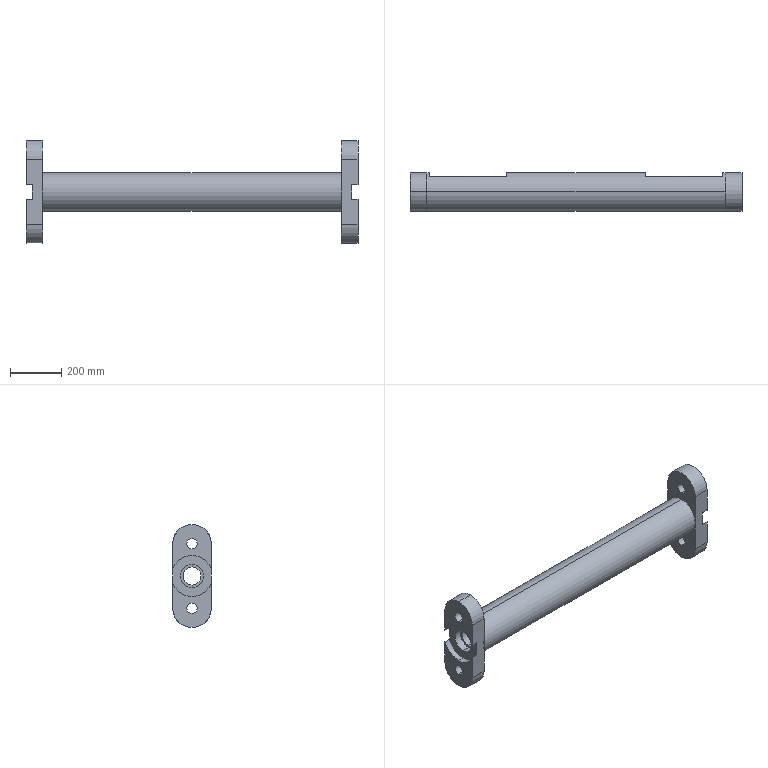Part | SolidWorks | features ICE 4, MirrorPattern 1, Revolution 1 | 1 solid | 58 faces | box 1290 x 150 x 400 mm | volume 20836949 mm3 | cylinder 36 | plane 22 | commonest cylinder face diameters 24 x8 40 x8 150 x8 160 x6 90 x4 70 x2